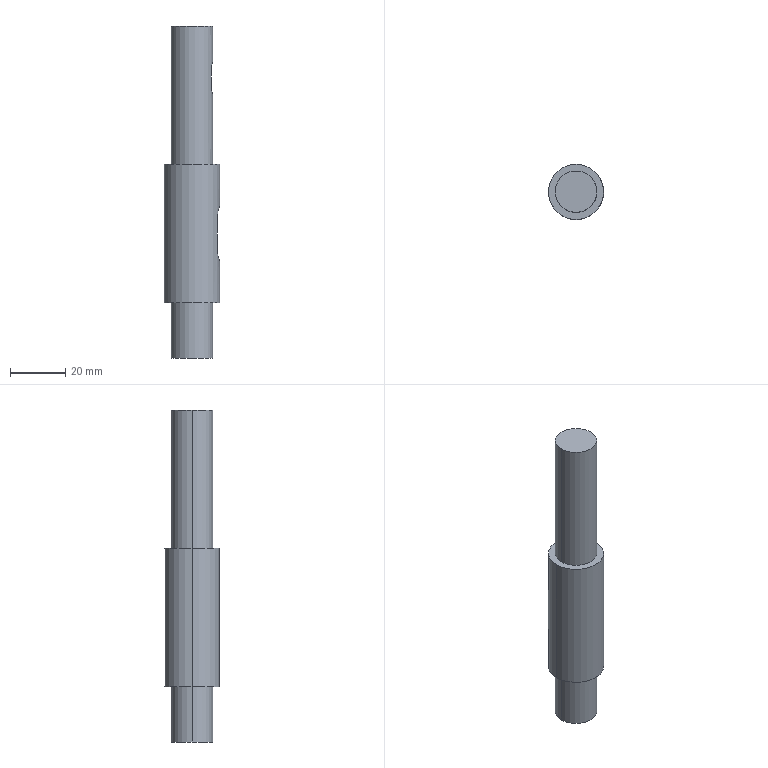Part | SolidWorks | features ICE 5, Extrusion 1 | 1 solid | 22 faces | box 20 x 20 x 120 mm | volume 27495 mm3 | cylinder 12 | plane 10 | commonest cylinder face diameters 15 x4 6 x3 8 x3 20 x2
STEP:
#1=CARTESIAN_POINT('',(-7.5,0.,-20.));
#2=VERTEX_POINT('',#1);
#3=CARTESIAN_POINT('',(7.5,0.,-20.));
#4=VERTEX_POINT('',#3);
#5=CARTESIAN_POINT('',(0.,0.,-20.));
#6=DIRECTION('',(0.,0.,-1.));
#7=DIRECTION('',(-1.,0.,0.));
#8=AXIS2_PLACEMENT_3D('',#5,#6,#7);
#9=CIRCLE('',#8,7.5);
#10=EDGE_CURVE('',#2,#4,#9,.T.);
#11=ORIENTED_EDGE('',*,*,#10,.F.);
#12=CARTESIAN_POINT('',(-7.5,0.,0.));
#13=VERTEX_POINT('',#12);
#14=CARTESIAN_POINT('',(-7.5,0.,-20.));
#15=DIRECTION('',(0.,0.,1.));
#16=VECTOR('',#15,1000.);
#17=LINE('',#14,#16);
#18=EDGE_CURVE('',#2,#13,#17,.T.);
#19=ORIENTED_EDGE('',*,*,#18,.T.);
#20=CARTESIAN_POINT('',(7.5,0.,0.));
#21=VERTEX_POINT('',#20);
#22=CARTESIAN_POINT('',(0.,0.,0.));
#23=DIRECTION('',(0.,0.,-1.));
#24=DIRECTION('',(-1.,0.,0.));
#25=AXIS2_PLACEMENT_3D('',#22,#23,#24);
#26=CIRCLE('',#25,7.5);
#27=EDGE_CURVE('',#13,#21,#26,.T.);
#28=ORIENTED_EDGE('',*,*,#27,.T.);
#29=CARTESIAN_POINT('',(7.5,0.,-20.));
#30=DIRECTION('',(0.,0.,1.));
#31=VECTOR('',#30,1000.);
#32=LINE('',#29,#31);
#33=EDGE_CURVE('',#4,#21,#32,.T.);
#34=ORIENTED_EDGE('',*,*,#33,.F.);
#35=EDGE_LOOP('',(#11,#19,#28,#34));
#36=FACE_OUTER_BOUND('',#35,.T.);
#37=CARTESIAN_POINT('',(0.,0.,-20.));
#38=DIRECTION('',(0.,0.,1.));
#39=DIRECTION('',(1.,0.,0.));
#40=AXIS2_PLACEMENT_3D('',#37,#38,#39);
#41=CYLINDRICAL_SURFACE('',#40,7.5);
#42=ADVANCED_FACE('',(#36),#41,.T.);
#43=CARTESIAN_POINT('',(4.5,0.,75.188));
#44=VERTEX_POINT('',#43);
#45=CARTESIAN_POINT('',(4.5,3.,78.188));
#46=VERTEX_POINT('',#45);
#47=CARTESIAN_POINT('',(4.5,0.,78.188));
#48=DIRECTION('',(1.,0.,0.));
#49=DIRECTION('',(0.,0.,-1.));
#50=AXIS2_PLACEMENT_3D('',#47,#48,#49);
#51=CIRCLE('',#50,3.);
#52=EDGE_CURVE('',#44,#46,#51,.T.);
#53=ORIENTED_EDGE('',*,*,#52,.F.);
#54=CARTESIAN_POINT('',(7.5,0.,75.188));
#55=VERTEX_POINT('',#54);
#56=CARTESIAN_POINT('',(4.5,0.,75.188));
#57=DIRECTION('',(1.,0.,0.));
#58=VECTOR('',#57,1000.);
#59=LINE('',#56,#58);
#60=EDGE_CURVE('',#44,#55,#59,.T.);
#61=ORIENTED_EDGE('',*,*,#60,.T.);
#62=CARTESIAN_POINT('',(6.874,3.,78.188));
#63=VERTEX_POINT('',#62);
#64=CARTESIAN_POINT('',(6.874,3.,78.188));
#65=CARTESIAN_POINT('',(6.874,3.,77.987));
#66=CARTESIAN_POINT('',(6.883,2.98,77.791));
#67=CARTESIAN_POINT('',(6.916,2.903,77.404));
#68=CARTESIAN_POINT('',(6.94,2.844,77.213));
#69=CARTESIAN_POINT('',(7.,2.693,76.851));
#70=CARTESIAN_POINT('',(7.036,2.6,76.679));
#71=CARTESIAN_POINT('',(7.112,2.383,76.355));
#72=CARTESIAN_POINT('',(7.154,2.258,76.203));
#73=CARTESIAN_POINT('',(7.275,1.847,75.792));
#74=CARTESIAN_POINT('',(7.354,1.515,75.57));
#75=CARTESIAN_POINT('',(7.439,0.9745,75.344));
#76=CARTESIAN_POINT('',(7.462,0.7831,75.285));
#77=CARTESIAN_POINT('',(7.492,0.3945,75.207));
#78=CARTESIAN_POINT('',(7.5,0.1982,75.188));
#79=CARTESIAN_POINT('',(7.5,0.,75.188));
#80=B_SPLINE_CURVE_WITH_KNOTS('',3,(#64,#65,#66,#67,#68,#69,#70,#71,#72,#73,#74,#75,#76,#77,#78,#79),.UNSPECIFIED.,.F.,.F.,(4,2,2,2,2,2,2,4),(0.,0.0005926,0.001185,0.001778,0.002371,0.003556,0.004148,0.004741),.UNSPECIFIED.);
#81=EDGE_CURVE('',#63,#55,#80,.T.);
#82=ORIENTED_EDGE('',*,*,#81,.F.);
#83=CARTESIAN_POINT('',(4.5,3.,78.188));
#84=DIRECTION('',(1.,0.,0.));
#85=VECTOR('',#84,1000.);
#86=LINE('',#83,#85);
#87=EDGE_CURVE('',#46,#63,#86,.T.);
#88=ORIENTED_EDGE('',*,*,#87,.F.);
#89=EDGE_LOOP('',(#53,#61,#82,#88));
#90=FACE_OUTER_BOUND('',#89,.T.);
#91=CARTESIAN_POINT('',(4.5,0.,78.188));
#92=DIRECTION('',(1.,0.,0.));
#93=DIRECTION('',(0.,0.,-1.));
#94=AXIS2_PLACEMENT_3D('',#91,#92,#93);
#95=CYLINDRICAL_SURFACE('',#94,3.);
#96=ADVANCED_FACE('',(#90),#95,.F.);
#97=CARTESIAN_POINT('',(7.5,0.,100.));
#98=VERTEX_POINT('',#97);
#99=CARTESIAN_POINT('',(-7.5,0.,100.));
#100=VERTEX_POINT('',#99);
#101=CARTESIAN_POINT('',(0.,0.,100.));
#102=DIRECTION('',(0.,0.,1.));
#103=DIRECTION('',(1.,0.,0.));
#104=AXIS2_PLACEMENT_3D('',#101,#102,#103);
#105=CIRCLE('',#104,7.5);
#106=EDGE_CURVE('',#98,#100,#105,.T.);
#107=ORIENTED_EDGE('',*,*,#106,.F.);
#108=CARTESIAN_POINT('',(7.5,0.,87.188));
#109=VERTEX_POINT('',#108);
#110=CARTESIAN_POINT('',(7.5,0.,100.));
#111=DIRECTION('',(0.,0.,-1.));
#112=VECTOR('',#111,1000.);
#113=LINE('',#110,#112);
#114=EDGE_CURVE('',#98,#109,#113,.T.);
#115=ORIENTED_EDGE('',*,*,#114,.T.);
#116=CARTESIAN_POINT('',(6.874,3.,84.188));
#117=VERTEX_POINT('',#116);
#118=CARTESIAN_POINT('',(7.5,0.,87.188));
#119=CARTESIAN_POINT('',(7.5,0.1979,87.188));
#120=CARTESIAN_POINT('',(7.492,0.3987,87.168));
#121=CARTESIAN_POINT('',(7.461,0.785,87.09));
#122=CARTESIAN_POINT('',(7.439,0.9732,87.033));
#123=CARTESIAN_POINT('',(7.382,1.339,86.88));
#124=CARTESIAN_POINT('',(7.348,1.51,86.787));
#125=CARTESIAN_POINT('',(7.274,1.833,86.571));
#126=CARTESIAN_POINT('',(7.234,1.985,86.445));
#127=CARTESIAN_POINT('',(7.153,2.26,86.171));
#128=CARTESIAN_POINT('',(7.113,2.382,86.022));
#129=CARTESIAN_POINT('',(7.036,2.599,85.698));
#130=CARTESIAN_POINT('',(7.,2.693,85.524));
#131=CARTESIAN_POINT('',(6.941,2.843,85.164));
#132=CARTESIAN_POINT('',(6.916,2.901,84.977));
#133=CARTESIAN_POINT('',(6.883,2.98,84.587));
#134=CARTESIAN_POINT('',(6.874,3.,84.388));
#135=CARTESIAN_POINT('',(6.874,3.,84.188));
#136=B_SPLINE_CURVE_WITH_KNOTS('',3,(#118,#119,#120,#121,#122,#123,#124,#125,#126,#127,#128,#129,#130,#131,#132,#133,#134,#135),.UNSPECIFIED.,.F.,.F.,(4,2,2,2,2,2,2,2,4),(0.004741,0.005333,0.005925,0.006516,0.007108,0.0077,0.008291,0.008883,0.009475),.UNSPECIFIED.);
#137=EDGE_CURVE('',#109,#117,#136,.T.);
#138=ORIENTED_EDGE('',*,*,#137,.T.);
#139=CARTESIAN_POINT('',(6.874,3.,100.));
#140=DIRECTION('',(0.,0.,-1.));
#141=VECTOR('',#140,1000.);
#142=LINE('',#139,#141);
#143=EDGE_CURVE('',#117,#63,#142,.T.);
#144=ORIENTED_EDGE('',*,*,#143,.T.);
#145=ORIENTED_EDGE('',*,*,#81,.T.);
#146=CARTESIAN_POINT('',(7.5,0.,50.));
#147=VERTEX_POINT('',#146);
#148=CARTESIAN_POINT('',(7.5,0.,100.));
#149=DIRECTION('',(0.,0.,-1.));
#150=VECTOR('',#149,1000.);
#151=LINE('',#148,#150);
#152=EDGE_CURVE('',#55,#147,#151,.T.);
#153=ORIENTED_EDGE('',*,*,#152,.T.);
#154=CARTESIAN_POINT('',(-7.5,0.,50.));
#155=VERTEX_POINT('',#154);
#156=CARTESIAN_POINT('',(0.,0.,50.));
#157=DIRECTION('',(0.,0.,1.));
#158=DIRECTION('',(1.,0.,0.));
#159=AXIS2_PLACEMENT_3D('',#156,#157,#158);
#160=CIRCLE('',#159,7.5);
#161=EDGE_CURVE('',#147,#155,#160,.T.);
#162=ORIENTED_EDGE('',*,*,#161,.T.);
#163=CARTESIAN_POINT('',(-7.5,0.,100.));
#164=DIRECTION('',(0.,0.,-1.));
#165=VECTOR('',#164,1000.);
#166=LINE('',#163,#165);
#167=EDGE_CURVE('',#100,#155,#166,.T.);
#168=ORIENTED_EDGE('',*,*,#167,.F.);
#169=EDGE_LOOP('',(#107,#115,#138,#144,#145,#153,#162,#168));
#170=FACE_OUTER_BOUND('',#169,.T.);
#171=CARTESIAN_POINT('',(0.,0.,100.));
#172=DIRECTION('',(0.,0.,-1.));
#173=DIRECTION('',(-1.,0.,0.));
#174=AXIS2_PLACEMENT_3D('',#171,#172,#173);
#175=CYLINDRICAL_SURFACE('',#174,7.5);
#176=ADVANCED_FACE('',(#170),#175,.T.);
#177=CARTESIAN_POINT('',(7.,0.,15.));
#178=VERTEX_POINT('',#177);
#179=CARTESIAN_POINT('',(7.,4.,19.));
#180=VERTEX_POINT('',#179);
#181=CARTESIAN_POINT('',(7.,0.,19.));
#182=DIRECTION('',(1.,0.,0.));
#183=DIRECTION('',(0.,0.,-1.));
#184=AXIS2_PLACEMENT_3D('',#181,#182,#183);
#185=CIRCLE('',#184,4.);
#186=EDGE_CURVE('',#178,#180,#185,.T.);
#187=ORIENTED_EDGE('',*,*,#186,.F.);
#188=CARTESIAN_POINT('',(10.,0.,15.));
#189=VERTEX_POINT('',#188);
#190=CARTESIAN_POINT('',(7.,0.,15.));
#191=DIRECTION('',(1.,0.,0.));
#192=VECTOR('',#191,1000.);
#193=LINE('',#190,#192);
#194=EDGE_CURVE('',#178,#189,#193,.T.);
#195=ORIENTED_EDGE('',*,*,#194,.T.);
#196=CARTESIAN_POINT('',(9.165,4.,19.));
#197=VERTEX_POINT('',#196);
#198=CARTESIAN_POINT('',(9.165,4.,19.));
#199=CARTESIAN_POINT('',(9.165,4.,18.733));
#200=CARTESIAN_POINT('',(9.177,3.973,18.47));
#201=CARTESIAN_POINT('',(9.221,3.87,17.955));
#202=CARTESIAN_POINT('',(9.254,3.792,17.7));
#203=CARTESIAN_POINT('',(9.334,3.59,17.217));
#204=CARTESIAN_POINT('',(9.381,3.467,16.988));
#205=CARTESIAN_POINT('',(9.483,3.177,16.555));
#206=CARTESIAN_POINT('',(9.538,3.01,16.353));
#207=CARTESIAN_POINT('',(9.646,2.645,15.988));
#208=CARTESIAN_POINT('',(9.699,2.444,15.823));
#209=CARTESIAN_POINT('',(9.799,2.009,15.531));
#210=CARTESIAN_POINT('',(9.843,1.78,15.409));
#211=CARTESIAN_POINT('',(9.918,1.299,15.208));
#212=CARTESIAN_POINT('',(9.949,1.044,15.13));
#213=CARTESIAN_POINT('',(9.99,0.526,15.026));
#214=CARTESIAN_POINT('',(10.,0.2643,15.));
#215=CARTESIAN_POINT('',(10.,0.,15.));
#216=B_SPLINE_CURVE_WITH_KNOTS('',3,(#198,#199,#200,#201,#202,#203,#204,#205,#206,#207,#208,#209,#210,#211,#212,#213,#214,#215),.UNSPECIFIED.,.F.,.F.,(4,2,2,2,2,2,2,2,4),(0.,0.0007902,0.00158,0.002371,0.003161,0.003951,0.004741,0.005531,0.006322),.UNSPECIFIED.);
#217=EDGE_CURVE('',#197,#189,#216,.T.);
#218=ORIENTED_EDGE('',*,*,#217,.F.);
#219=CARTESIAN_POINT('',(7.,4.,19.));
#220=DIRECTION('',(1.,0.,0.));
#221=VECTOR('',#220,1000.);
#222=LINE('',#219,#221);
#223=EDGE_CURVE('',#180,#197,#222,.T.);
#224=ORIENTED_EDGE('',*,*,#223,.F.);
#225=EDGE_LOOP('',(#187,#195,#218,#224));
#226=FACE_OUTER_BOUND('',#225,.T.);
#227=CARTESIAN_POINT('',(7.,0.,19.));
#228=DIRECTION('',(1.,0.,0.));
#229=DIRECTION('',(0.,0.,-1.));
#230=AXIS2_PLACEMENT_3D('',#227,#228,#229);
#231=CYLINDRICAL_SURFACE('',#230,4.);
#232=ADVANCED_FACE('',(#226),#231,.F.);
#233=CARTESIAN_POINT('',(10.,0.,50.));
#234=VERTEX_POINT('',#233);
#235=CARTESIAN_POINT('',(-10.,0.,50.));
#236=VERTEX_POINT('',#235);
#237=CARTESIAN_POINT('',(0.,0.,50.));
#238=DIRECTION('',(0.,0.,1.));
#239=DIRECTION('',(1.,0.,0.));
#240=AXIS2_PLACEMENT_3D('',#237,#238,#239);
#241=CIRCLE('',#240,10.);
#242=EDGE_CURVE('',#234,#236,#241,.T.);
#243=ORIENTED_EDGE('',*,*,#242,.F.);
#244=CARTESIAN_POINT('',(10.,0.,35.));
#245=VERTEX_POINT('',#244);
#246=CARTESIAN_POINT('',(10.,0.,60.));
#247=DIRECTION('',(0.,0.,-1.));
#248=VECTOR('',#247,1000.);
#249=LINE('',#246,#248);
#250=EDGE_CURVE('',#234,#245,#249,.T.);
#251=ORIENTED_EDGE('',*,*,#250,.T.);
#252=CARTESIAN_POINT('',(9.165,4.,31.));
#253=VERTEX_POINT('',#252);
#254=CARTESIAN_POINT('',(10.,0.,35.));
#255=CARTESIAN_POINT('',(10.,0.2639,35.));
#256=CARTESIAN_POINT('',(9.989,0.5316,34.973));
#257=CARTESIAN_POINT('',(9.948,1.047,34.87));
#258=CARTESIAN_POINT('',(9.919,1.298,34.793));
#259=CARTESIAN_POINT('',(9.843,1.785,34.589));
#260=CARTESIAN_POINT('',(9.798,2.014,34.466));
#261=CARTESIAN_POINT('',(9.699,2.444,34.177));
#262=CARTESIAN_POINT('',(9.645,2.647,34.01));
#263=CARTESIAN_POINT('',(9.537,3.013,33.644));
#264=CARTESIAN_POINT('',(9.483,3.176,33.445));
#265=CARTESIAN_POINT('',(9.381,3.466,33.014));
#266=CARTESIAN_POINT('',(9.334,3.591,32.781));
#267=CARTESIAN_POINT('',(9.254,3.791,32.302));
#268=CARTESIAN_POINT('',(9.222,3.868,32.052));
#269=CARTESIAN_POINT('',(9.177,3.973,31.533));
#270=CARTESIAN_POINT('',(9.165,4.,31.267));
#271=CARTESIAN_POINT('',(9.165,4.,31.));
#272=B_SPLINE_CURVE_WITH_KNOTS('',3,(#254,#255,#256,#257,#258,#259,#260,#261,#262,#263,#264,#265,#266,#267,#268,#269,#270,#271),.UNSPECIFIED.,.F.,.F.,(4,2,2,2,2,2,2,2,4),(0.006322,0.00711,0.007899,0.008688,0.009477,0.01027,0.01106,0.01184,0.01263),.UNSPECIFIED.);
#273=EDGE_CURVE('',#245,#253,#272,.T.);
#274=ORIENTED_EDGE('',*,*,#273,.T.);
#275=CARTESIAN_POINT('',(9.165,4.,60.));
#276=DIRECTION('',(0.,0.,-1.));
#277=VECTOR('',#276,1000.);
#278=LINE('',#275,#277);
#279=EDGE_CURVE('',#253,#197,#278,.T.);
#280=ORIENTED_EDGE('',*,*,#279,.T.);
#281=ORIENTED_EDGE('',*,*,#217,.T.);
#282=CARTESIAN_POINT('',(10.,0.,0.));
#283=VERTEX_POINT('',#282);
#284=CARTESIAN_POINT('',(10.,0.,60.));
#285=DIRECTION('',(0.,0.,-1.));
#286=VECTOR('',#285,1000.);
#287=LINE('',#284,#286);
#288=EDGE_CURVE('',#189,#283,#287,.T.);
#289=ORIENTED_EDGE('',*,*,#288,.T.);
#290=CARTESIAN_POINT('',(-10.,0.,0.));
#291=VERTEX_POINT('',#290);
#292=CARTESIAN_POINT('',(0.,0.,0.));
#293=DIRECTION('',(0.,0.,1.));
#294=DIRECTION('',(1.,0.,0.));
#295=AXIS2_PLACEMENT_3D('',#292,#293,#294);
#296=CIRCLE('',#295,10.);
#297=EDGE_CURVE('',#283,#291,#296,.T.);
#298=ORIENTED_EDGE('',*,*,#297,.T.);
#299=CARTESIAN_POINT('',(-10.,0.,60.));
#300=DIRECTION('',(0.,0.,-1.));
#301=VECTOR('',#300,1000.);
#302=LINE('',#299,#301);
#303=EDGE_CURVE('',#236,#291,#302,.T.);
#304=ORIENTED_EDGE('',*,*,#303,.F.);
#305=EDGE_LOOP('',(#243,#251,#274,#280,#281,#289,#298,#304));
#306=FACE_OUTER_BOUND('',#305,.T.);
#307=CARTESIAN_POINT('',(0.,0.,60.));
#308=DIRECTION('',(0.,0.,-1.));
#309=DIRECTION('',(-1.,0.,0.));
#310=AXIS2_PLACEMENT_3D('',#307,#308,#309);
#311=CYLINDRICAL_SURFACE('',#310,10.);
#312=ADVANCED_FACE('',(#306),#311,.T.);
#313=ORIENTED_EDGE('',*,*,#250,.F.);
#314=CARTESIAN_POINT('',(0.,0.,50.));
#315=DIRECTION('',(0.,0.,1.));
#316=DIRECTION('',(1.,0.,0.));
#317=AXIS2_PLACEMENT_3D('',#314,#315,#316);
#318=CIRCLE('',#317,10.);
#319=EDGE_CURVE('',#236,#234,#318,.T.);
#320=ORIENTED_EDGE('',*,*,#319,.F.);
#321=ORIENTED_EDGE('',*,*,#303,.T.);
#322=CARTESIAN_POINT('',(0.,0.,0.));
#323=DIRECTION('',(0.,0.,1.));
#324=DIRECTION('',(1.,0.,0.));
#325=AXIS2_PLACEMENT_3D('',#322,#323,#324);
#326=CIRCLE('',#325,10.);
#327=EDGE_CURVE('',#291,#283,#326,.T.);
#328=ORIENTED_EDGE('',*,*,#327,.T.);
#329=ORIENTED_EDGE('',*,*,#288,.F.);
#330=CARTESIAN_POINT('',(9.165,-4.,19.));
#331=VERTEX_POINT('',#330);
#332=CARTESIAN_POINT('',(10.,0.,15.));
#333=CARTESIAN_POINT('',(10.,-0.2639,15.));
#334=CARTESIAN_POINT('',(9.989,-0.5316,15.027));
#335=CARTESIAN_POINT('',(9.948,-1.047,15.13));
#336=CARTESIAN_POINT('',(9.919,-1.298,15.207));
#337=CARTESIAN_POINT('',(9.843,-1.785,15.411));
#338=CARTESIAN_POINT('',(9.798,-2.014,15.534));
#339=CARTESIAN_POINT('',(9.699,-2.444,15.823));
#340=CARTESIAN_POINT('',(9.645,-2.647,15.99));
#341=CARTESIAN_POINT('',(9.537,-3.013,16.356));
#342=CARTESIAN_POINT('',(9.483,-3.176,16.555));
#343=CARTESIAN_POINT('',(9.381,-3.466,16.986));
#344=CARTESIAN_POINT('',(9.334,-3.591,17.219));
#345=CARTESIAN_POINT('',(9.254,-3.791,17.698));
#346=CARTESIAN_POINT('',(9.222,-3.868,17.948));
#347=CARTESIAN_POINT('',(9.177,-3.973,18.467));
#348=CARTESIAN_POINT('',(9.165,-4.,18.733));
#349=CARTESIAN_POINT('',(9.165,-4.,19.));
#350=B_SPLINE_CURVE_WITH_KNOTS('',3,(#332,#333,#334,#335,#336,#337,#338,#339,#340,#341,#342,#343,#344,#345,#346,#347,#348,#349),.UNSPECIFIED.,.F.,.F.,(4,2,2,2,2,2,2,2,4),(0.006322,0.00711,0.007899,0.008688,0.009477,0.01027,0.01106,0.01184,0.01263),.UNSPECIFIED.);
#351=EDGE_CURVE('',#189,#331,#350,.T.);
#352=ORIENTED_EDGE('',*,*,#351,.T.);
#353=CARTESIAN_POINT('',(9.165,-4.,31.));
#354=VERTEX_POINT('',#353);
#355=CARTESIAN_POINT('',(9.165,-4.,60.));
#356=DIRECTION('',(0.,0.,1.));
#357=VECTOR('',#356,1000.);
#358=LINE('',#355,#357);
#359=EDGE_CURVE('',#331,#354,#358,.T.);
#360=ORIENTED_EDGE('',*,*,#359,.T.);
#361=CARTESIAN_POINT('',(9.165,-4.,31.));
#362=CARTESIAN_POINT('',(9.165,-4.,31.267));
#363=CARTESIAN_POINT('',(9.177,-3.973,31.53));
#364=CARTESIAN_POINT('',(9.221,-3.87,32.045));
#365=CARTESIAN_POINT('',(9.254,-3.792,32.3));
#366=CARTESIAN_POINT('',(9.334,-3.59,32.783));
#367=CARTESIAN_POINT('',(9.381,-3.467,33.012));
#368=CARTESIAN_POINT('',(9.483,-3.177,33.445));
#369=CARTESIAN_POINT('',(9.538,-3.01,33.647));
#370=CARTESIAN_POINT('',(9.646,-2.645,34.012));
#371=CARTESIAN_POINT('',(9.699,-2.444,34.177));
#372=CARTESIAN_POINT('',(9.799,-2.009,34.469));
#373=CARTESIAN_POINT('',(9.843,-1.78,34.591));
#374=CARTESIAN_POINT('',(9.918,-1.299,34.792));
#375=CARTESIAN_POINT('',(9.949,-1.044,34.87));
#376=CARTESIAN_POINT('',(9.99,-0.526,34.974));
#377=CARTESIAN_POINT('',(10.,-0.2643,35.));
#378=CARTESIAN_POINT('',(10.,0.,35.));
#379=B_SPLINE_CURVE_WITH_KNOTS('',3,(#361,#362,#363,#364,#365,#366,#367,#368,#369,#370,#371,#372,#373,#374,#375,#376,#377,#378),.UNSPECIFIED.,.F.,.F.,(4,2,2,2,2,2,2,2,4),(0.,0.0007902,0.00158,0.002371,0.003161,0.003951,0.004741,0.005531,0.006322),.UNSPECIFIED.);
#380=EDGE_CURVE('',#354,#245,#379,.T.);
#381=ORIENTED_EDGE('',*,*,#380,.T.);
#382=EDGE_LOOP('',(#313,#320,#321,#328,#329,#352,#360,#381));
#383=FACE_OUTER_BOUND('',#382,.T.);
#384=CARTESIAN_POINT('',(0.,0.,60.));
#385=DIRECTION('',(0.,0.,-1.));
#386=DIRECTION('',(-1.,0.,0.));
#387=AXIS2_PLACEMENT_3D('',#384,#385,#386);
#388=CYLINDRICAL_SURFACE('',#387,10.);
#389=ADVANCED_FACE('',(#383),#388,.T.);
#390=CARTESIAN_POINT('',(0.,0.,0.));
#391=DIRECTION('',(0.,0.,-1.));
#392=DIRECTION('',(-1.,0.,0.));
#393=AXIS2_PLACEMENT_3D('',#390,#391,#392);
#394=CIRCLE('',#393,7.5);
#395=EDGE_CURVE('',#21,#13,#394,.T.);
#396=ORIENTED_EDGE('',*,*,#395,.F.);
#397=ORIENTED_EDGE('',*,*,#27,.F.);
#398=EDGE_LOOP('',(#396,#397));
#399=FACE_BOUND('',#398,.T.);
#400=ORIENTED_EDGE('',*,*,#327,.F.);
#401=ORIENTED_EDGE('',*,*,#297,.F.);
#402=EDGE_LOOP('',(#400,#401));
#403=FACE_OUTER_BOUND('',#402,.T.);
#404=CARTESIAN_POINT('',(0.,0.,0.));
#405=DIRECTION('',(0.,0.,1.));
#406=DIRECTION('',(1.,0.,0.));
#407=AXIS2_PLACEMENT_3D('',#404,#405,#406);
#408=PLANE('',#407);
#409=ADVANCED_FACE('',(#399,#403),#408,.F.);
#410=CARTESIAN_POINT('',(7.,-4.,31.));
#411=VERTEX_POINT('',#410);
#412=CARTESIAN_POINT('',(7.,-4.,31.));
#413=DIRECTION('',(1.,0.,0.));
#414=VECTOR('',#413,1000.);
#415=LINE('',#412,#414);
#416=EDGE_CURVE('',#411,#354,#415,.T.);
#417=ORIENTED_EDGE('',*,*,#416,.F.);
#418=CARTESIAN_POINT('',(7.,4.,31.));
#419=VERTEX_POINT('',#418);
#420=CARTESIAN_POINT('',(7.,0.,31.));
#421=DIRECTION('',(1.,0.,0.));
#422=DIRECTION('',(0.,0.,-1.));
#423=AXIS2_PLACEMENT_3D('',#420,#421,#422);
#424=CIRCLE('',#423,4.);
#425=EDGE_CURVE('',#419,#411,#424,.T.);
#426=ORIENTED_EDGE('',*,*,#425,.F.);
#427=CARTESIAN_POINT('',(7.,4.,31.));
#428=DIRECTION('',(1.,0.,0.));
#429=VECTOR('',#428,1000.);
#430=LINE('',#427,#429);
#431=EDGE_CURVE('',#419,#253,#430,.T.);
#432=ORIENTED_EDGE('',*,*,#431,.T.);
#433=ORIENTED_EDGE('',*,*,#273,.F.);
#434=ORIENTED_EDGE('',*,*,#380,.F.);
#435=EDGE_LOOP('',(#417,#426,#432,#433,#434));
#436=FACE_OUTER_BOUND('',#435,.T.);
#437=CARTESIAN_POINT('',(7.,0.,31.));
#438=DIRECTION('',(1.,0.,0.));
#439=DIRECTION('',(0.,0.,-1.));
#440=AXIS2_PLACEMENT_3D('',#437,#438,#439);
#441=CYLINDRICAL_SURFACE('',#440,4.);
#442=ADVANCED_FACE('',(#436),#441,.F.);
#443=ORIENTED_EDGE('',*,*,#431,.F.);
#444=CARTESIAN_POINT('',(7.,4.,31.));
#445=DIRECTION('',(0.,0.,1.));
#446=VECTOR('',#445,1000.);
#447=LINE('',#444,#446);
#448=EDGE_CURVE('',#180,#419,#447,.T.);
#449=ORIENTED_EDGE('',*,*,#448,.F.);
#450=ORIENTED_EDGE('',*,*,#223,.T.);
#451=ORIENTED_EDGE('',*,*,#279,.F.);
#452=EDGE_LOOP('',(#443,#449,#450,#451));
#453=FACE_OUTER_BOUND('',#452,.T.);
#454=CARTESIAN_POINT('',(7.,4.,31.));
#455=DIRECTION('',(0.,1.,0.));
#456=DIRECTION('',(0.,0.,1.));
#457=AXIS2_PLACEMENT_3D('',#454,#455,#456);
#458=PLANE('',#457);
#459=ADVANCED_FACE('',(#453),#458,.F.);
#460=ORIENTED_EDGE('',*,*,#194,.F.);
#461=CARTESIAN_POINT('',(7.,-4.,19.));
#462=VERTEX_POINT('',#461);
#463=CARTESIAN_POINT('',(7.,0.,19.));
#464=DIRECTION('',(1.,0.,0.));
#465=DIRECTION('',(0.,0.,-1.));
#466=AXIS2_PLACEMENT_3D('',#463,#464,#465);
#467=CIRCLE('',#466,4.);
#468=EDGE_CURVE('',#462,#178,#467,.T.);
#469=ORIENTED_EDGE('',*,*,#468,.F.);
#470=CARTESIAN_POINT('',(7.,-4.,19.));
#471=DIRECTION('',(1.,0.,0.));
#472=VECTOR('',#471,1000.);
#473=LINE('',#470,#472);
#474=EDGE_CURVE('',#462,#331,#473,.T.);
#475=ORIENTED_EDGE('',*,*,#474,.T.);
#476=ORIENTED_EDGE('',*,*,#351,.F.);
#477=EDGE_LOOP('',(#460,#469,#475,#476));
#478=FACE_OUTER_BOUND('',#477,.T.);
#479=CARTESIAN_POINT('',(7.,0.,19.));
#480=DIRECTION('',(1.,0.,0.));
#481=DIRECTION('',(0.,0.,-1.));
#482=AXIS2_PLACEMENT_3D('',#479,#480,#481);
#483=CYLINDRICAL_SURFACE('',#482,4.);
#484=ADVANCED_FACE('',(#478),#483,.F.);
#485=ORIENTED_EDGE('',*,*,#474,.F.);
#486=CARTESIAN_POINT('',(7.,-4.,31.));
#487=DIRECTION('',(0.,0.,-1.));
#488=VECTOR('',#487,1000.);
#489=LINE('',#486,#488);
#490=EDGE_CURVE('',#411,#462,#489,.T.);
#491=ORIENTED_EDGE('',*,*,#490,.F.);
#492=ORIENTED_EDGE('',*,*,#416,.T.);
#493=ORIENTED_EDGE('',*,*,#359,.F.);
#494=EDGE_LOOP('',(#485,#491,#492,#493));
#495=FACE_OUTER_BOUND('',#494,.T.);
#496=CARTESIAN_POINT('',(7.,-4.,31.));
#497=DIRECTION('',(0.,-1.,0.));
#498=DIRECTION('',(0.,0.,-1.));
#499=AXIS2_PLACEMENT_3D('',#496,#497,#498);
#500=PLANE('',#499);
#501=ADVANCED_FACE('',(#495),#500,.F.);
#502=ORIENTED_EDGE('',*,*,#425,.T.);
#503=ORIENTED_EDGE('',*,*,#490,.T.);
#504=ORIENTED_EDGE('',*,*,#468,.T.);
#505=ORIENTED_EDGE('',*,*,#186,.T.);
#506=ORIENTED_EDGE('',*,*,#448,.T.);
#507=EDGE_LOOP('',(#502,#503,#504,#505,#506));
#508=FACE_OUTER_BOUND('',#507,.T.);
#509=CARTESIAN_POINT('',(7.,0.,31.));
#510=DIRECTION('',(1.,0.,0.));
#511=DIRECTION('',(0.,0.,-1.));
#512=AXIS2_PLACEMENT_3D('',#509,#510,#511);
#513=PLANE('',#512);
#514=ADVANCED_FACE('',(#508),#513,.T.);
#515=CARTESIAN_POINT('',(0.,0.,50.));
#516=DIRECTION('',(0.,0.,1.));
#517=DIRECTION('',(1.,0.,0.));
#518=AXIS2_PLACEMENT_3D('',#515,#516,#517);
#519=CIRCLE('',#518,7.5);
#520=EDGE_CURVE('',#155,#147,#519,.T.);
#521=ORIENTED_EDGE('',*,*,#520,.F.);
#522=ORIENTED_EDGE('',*,*,#161,.F.);
#523=EDGE_LOOP('',(#521,#522));
#524=FACE_BOUND('',#523,.T.);
#525=ORIENTED_EDGE('',*,*,#319,.T.);
#526=ORIENTED_EDGE('',*,*,#242,.T.);
#527=EDGE_LOOP('',(#525,#526));
#528=FACE_OUTER_BOUND('',#527,.T.);
#529=CARTESIAN_POINT('',(0.,0.,50.));
#530=DIRECTION('',(0.,0.,1.));
#531=DIRECTION('',(1.,0.,0.));
#532=AXIS2_PLACEMENT_3D('',#529,#530,#531);
#533=PLANE('',#532);
#534=ADVANCED_FACE('',(#524,#528),#533,.T.);
#535=CARTESIAN_POINT('',(0.,0.,100.));
#536=DIRECTION('',(0.,0.,1.));
#537=DIRECTION('',(1.,0.,0.));
#538=AXIS2_PLACEMENT_3D('',#535,#536,#537);
#539=CIRCLE('',#538,7.5);
#540=EDGE_CURVE('',#100,#98,#539,.T.);
#541=ORIENTED_EDGE('',*,*,#540,.T.);
#542=ORIENTED_EDGE('',*,*,#106,.T.);
#543=EDGE_LOOP('',(#541,#542));
#544=FACE_OUTER_BOUND('',#543,.T.);
#545=CARTESIAN_POINT('',(0.,0.,100.));
#546=DIRECTION('',(0.,0.,1.));
#547=DIRECTION('',(1.,0.,0.));
#548=AXIS2_PLACEMENT_3D('',#545,#546,#547);
#549=PLANE('',#548);
#550=ADVANCED_FACE('',(#544),#549,.T.);
#551=ORIENTED_EDGE('',*,*,#114,.F.);
#552=ORIENTED_EDGE('',*,*,#540,.F.);
#553=ORIENTED_EDGE('',*,*,#167,.T.);
#554=ORIENTED_EDGE('',*,*,#520,.T.);
#555=ORIENTED_EDGE('',*,*,#152,.F.);
#556=CARTESIAN_POINT('',(6.874,-3.,78.188));
#557=VERTEX_POINT('',#556);
#558=CARTESIAN_POINT('',(7.5,0.,75.188));
#559=CARTESIAN_POINT('',(7.5,-0.1979,75.188));
#560=CARTESIAN_POINT('',(7.492,-0.3987,75.208));
#561=CARTESIAN_POINT('',(7.461,-0.785,75.286));
#562=CARTESIAN_POINT('',(7.439,-0.9732,75.343));
#563=CARTESIAN_POINT('',(7.382,-1.339,75.496));
#564=CARTESIAN_POINT('',(7.348,-1.51,75.589));
#565=CARTESIAN_POINT('',(7.274,-1.833,75.805));
#566=CARTESIAN_POINT('',(7.234,-1.985,75.931));
#567=CARTESIAN_POINT('',(7.153,-2.26,76.205));
#568=CARTESIAN_POINT('',(7.113,-2.382,76.354));
#569=CARTESIAN_POINT('',(7.036,-2.599,76.678));
#570=CARTESIAN_POINT('',(7.,-2.693,76.852));
#571=CARTESIAN_POINT('',(6.941,-2.843,77.212));
#572=CARTESIAN_POINT('',(6.916,-2.901,77.399));
#573=CARTESIAN_POINT('',(6.883,-2.98,77.789));
#574=CARTESIAN_POINT('',(6.874,-3.,77.988));
#575=CARTESIAN_POINT('',(6.874,-3.,78.188));
#576=B_SPLINE_CURVE_WITH_KNOTS('',3,(#558,#559,#560,#561,#562,#563,#564,#565,#566,#567,#568,#569,#570,#571,#572,#573,#574,#575),.UNSPECIFIED.,.F.,.F.,(4,2,2,2,2,2,2,2,4),(0.004741,0.005333,0.005925,0.006516,0.007108,0.0077,0.008291,0.008883,0.009475),.UNSPECIFIED.);
#577=EDGE_CURVE('',#55,#557,#576,.T.);
#578=ORIENTED_EDGE('',*,*,#577,.T.);
#579=CARTESIAN_POINT('',(6.874,-3.,84.188));
#580=VERTEX_POINT('',#579);
#581=CARTESIAN_POINT('',(6.874,-3.,100.));
#582=DIRECTION('',(0.,0.,1.));
#583=VECTOR('',#582,1000.);
#584=LINE('',#581,#583);
#585=EDGE_CURVE('',#557,#580,#584,.T.);
#586=ORIENTED_EDGE('',*,*,#585,.T.);
#587=CARTESIAN_POINT('',(6.874,-3.,84.188));
#588=CARTESIAN_POINT('',(6.874,-3.,84.389));
#589=CARTESIAN_POINT('',(6.883,-2.98,84.585));
#590=CARTESIAN_POINT('',(6.916,-2.903,84.972));
#591=CARTESIAN_POINT('',(6.94,-2.844,85.163));
#592=CARTESIAN_POINT('',(7.,-2.693,85.525));
#593=CARTESIAN_POINT('',(7.036,-2.6,85.697));
#594=CARTESIAN_POINT('',(7.112,-2.383,86.021));
#595=CARTESIAN_POINT('',(7.154,-2.258,86.173));
#596=CARTESIAN_POINT('',(7.275,-1.847,86.584));
#597=CARTESIAN_POINT('',(7.354,-1.515,86.806));
#598=CARTESIAN_POINT('',(7.439,-0.9745,87.032));
#599=CARTESIAN_POINT('',(7.462,-0.7831,87.091));
#600=CARTESIAN_POINT('',(7.492,-0.3945,87.169));
#601=CARTESIAN_POINT('',(7.5,-0.1982,87.188));
#602=CARTESIAN_POINT('',(7.5,0.,87.188));
#603=B_SPLINE_CURVE_WITH_KNOTS('',3,(#587,#588,#589,#590,#591,#592,#593,#594,#595,#596,#597,#598,#599,#600,#601,#602),.UNSPECIFIED.,.F.,.F.,(4,2,2,2,2,2,2,4),(0.,0.0005926,0.001185,0.001778,0.002371,0.003556,0.004148,0.004741),.UNSPECIFIED.);
#604=EDGE_CURVE('',#580,#109,#603,.T.);
#605=ORIENTED_EDGE('',*,*,#604,.T.);
#606=EDGE_LOOP('',(#551,#552,#553,#554,#555,#578,#586,#605));
#607=FACE_OUTER_BOUND('',#606,.T.);
#608=CARTESIAN_POINT('',(0.,0.,100.));
#609=DIRECTION('',(0.,0.,-1.));
#610=DIRECTION('',(-1.,0.,0.));
#611=AXIS2_PLACEMENT_3D('',#608,#609,#610);
#612=CYLINDRICAL_SURFACE('',#611,7.5);
#613=ADVANCED_FACE('',(#607),#612,.T.);
#614=CARTESIAN_POINT('',(4.5,-3.,84.188));
#615=VERTEX_POINT('',#614);
#616=CARTESIAN_POINT('',(4.5,-3.,84.188));
#617=DIRECTION('',(1.,0.,0.));
#618=VECTOR('',#617,1000.);
#619=LINE('',#616,#618);
#620=EDGE_CURVE('',#615,#580,#619,.T.);
#621=ORIENTED_EDGE('',*,*,#620,.F.);
#622=CARTESIAN_POINT('',(4.5,3.,84.188));
#623=VERTEX_POINT('',#622);
#624=CARTESIAN_POINT('',(4.5,0.,84.188));
#625=DIRECTION('',(1.,0.,0.));
#626=DIRECTION('',(0.,0.,-1.));
#627=AXIS2_PLACEMENT_3D('',#624,#625,#626);
#628=CIRCLE('',#627,3.);
#629=EDGE_CURVE('',#623,#615,#628,.T.);
#630=ORIENTED_EDGE('',*,*,#629,.F.);
#631=CARTESIAN_POINT('',(4.5,3.,84.188));
#632=DIRECTION('',(1.,0.,0.));
#633=VECTOR('',#632,1000.);
#634=LINE('',#631,#633);
#635=EDGE_CURVE('',#623,#117,#634,.T.);
#636=ORIENTED_EDGE('',*,*,#635,.T.);
#637=ORIENTED_EDGE('',*,*,#137,.F.);
#638=ORIENTED_EDGE('',*,*,#604,.F.);
#639=EDGE_LOOP('',(#621,#630,#636,#637,#638));
#640=FACE_OUTER_BOUND('',#639,.T.);
#641=CARTESIAN_POINT('',(4.5,0.,84.188));
#642=DIRECTION('',(1.,0.,0.));
#643=DIRECTION('',(0.,0.,-1.));
#644=AXIS2_PLACEMENT_3D('',#641,#642,#643);
#645=CYLINDRICAL_SURFACE('',#644,3.);
#646=ADVANCED_FACE('',(#640),#645,.F.);
#647=ORIENTED_EDGE('',*,*,#635,.F.);
#648=CARTESIAN_POINT('',(4.5,3.,84.188));
#649=DIRECTION('',(0.,0.,1.));
#650=VECTOR('',#649,1000.);
#651=LINE('',#648,#650);
#652=EDGE_CURVE('',#46,#623,#651,.T.);
#653=ORIENTED_EDGE('',*,*,#652,.F.);
#654=ORIENTED_EDGE('',*,*,#87,.T.);
#655=ORIENTED_EDGE('',*,*,#143,.F.);
#656=EDGE_LOOP('',(#647,#653,#654,#655));
#657=FACE_OUTER_BOUND('',#656,.T.);
#658=CARTESIAN_POINT('',(4.5,3.,84.188));
#659=DIRECTION('',(0.,1.,0.));
#660=DIRECTION('',(0.,0.,1.));
#661=AXIS2_PLACEMENT_3D('',#658,#659,#660);
#662=PLANE('',#661);
#663=ADVANCED_FACE('',(#657),#662,.F.);
#664=ORIENTED_EDGE('',*,*,#60,.F.);
#665=CARTESIAN_POINT('',(4.5,-3.,78.188));
#666=VERTEX_POINT('',#665);
#667=CARTESIAN_POINT('',(4.5,0.,78.188));
#668=DIRECTION('',(1.,0.,0.));
#669=DIRECTION('',(0.,0.,-1.));
#670=AXIS2_PLACEMENT_3D('',#667,#668,#669);
#671=CIRCLE('',#670,3.);
#672=EDGE_CURVE('',#666,#44,#671,.T.);
#673=ORIENTED_EDGE('',*,*,#672,.F.);
#674=CARTESIAN_POINT('',(4.5,-3.,78.188));
#675=DIRECTION('',(1.,0.,0.));
#676=VECTOR('',#675,1000.);
#677=LINE('',#674,#676);
#678=EDGE_CURVE('',#666,#557,#677,.T.);
#679=ORIENTED_EDGE('',*,*,#678,.T.);
#680=ORIENTED_EDGE('',*,*,#577,.F.);
#681=EDGE_LOOP('',(#664,#673,#679,#680));
#682=FACE_OUTER_BOUND('',#681,.T.);
#683=CARTESIAN_POINT('',(4.5,0.,78.188));
#684=DIRECTION('',(1.,0.,0.));
#685=DIRECTION('',(0.,0.,-1.));
#686=AXIS2_PLACEMENT_3D('',#683,#684,#685);
#687=CYLINDRICAL_SURFACE('',#686,3.);
#688=ADVANCED_FACE('',(#682),#687,.F.);
#689=ORIENTED_EDGE('',*,*,#678,.F.);
#690=CARTESIAN_POINT('',(4.5,-3.,84.188));
#691=DIRECTION('',(0.,0.,-1.));
#692=VECTOR('',#691,1000.);
#693=LINE('',#690,#692);
#694=EDGE_CURVE('',#615,#666,#693,.T.);
#695=ORIENTED_EDGE('',*,*,#694,.F.);
#696=ORIENTED_EDGE('',*,*,#620,.T.);
#697=ORIENTED_EDGE('',*,*,#585,.F.);
#698=EDGE_LOOP('',(#689,#695,#696,#697));
#699=FACE_OUTER_BOUND('',#698,.T.);
#700=CARTESIAN_POINT('',(4.5,-3.,84.188));
#701=DIRECTION('',(0.,-1.,0.));
#702=DIRECTION('',(0.,0.,-1.));
#703=AXIS2_PLACEMENT_3D('',#700,#701,#702);
#704=PLANE('',#703);
#705=ADVANCED_FACE('',(#699),#704,.F.);
#706=ORIENTED_EDGE('',*,*,#629,.T.);
#707=ORIENTED_EDGE('',*,*,#694,.T.);
#708=ORIENTED_EDGE('',*,*,#672,.T.);
#709=ORIENTED_EDGE('',*,*,#52,.T.);
#710=ORIENTED_EDGE('',*,*,#652,.T.);
#711=EDGE_LOOP('',(#706,#707,#708,#709,#710));
#712=FACE_OUTER_BOUND('',#711,.T.);
#713=CARTESIAN_POINT('',(4.5,0.,84.188));
#714=DIRECTION('',(1.,0.,0.));
#715=DIRECTION('',(0.,0.,-1.));
#716=AXIS2_PLACEMENT_3D('',#713,#714,#715);
#717=PLANE('',#716);
#718=ADVANCED_FACE('',(#712),#717,.T.);
#719=ORIENTED_EDGE('',*,*,#18,.F.);
#720=CARTESIAN_POINT('',(0.,0.,-20.));
#721=DIRECTION('',(0.,0.,-1.));
#722=DIRECTION('',(-1.,0.,0.));
#723=AXIS2_PLACEMENT_3D('',#720,#721,#722);
#724=CIRCLE('',#723,7.5);
#725=EDGE_CURVE('',#4,#2,#724,.T.);
#726=ORIENTED_EDGE('',*,*,#725,.F.);
#727=ORIENTED_EDGE('',*,*,#33,.T.);
#728=ORIENTED_EDGE('',*,*,#395,.T.);
#729=EDGE_LOOP('',(#719,#726,#727,#728));
#730=FACE_OUTER_BOUND('',#729,.T.);
#731=CARTESIAN_POINT('',(0.,0.,-20.));
#732=DIRECTION('',(0.,0.,1.));
#733=DIRECTION('',(1.,0.,0.));
#734=AXIS2_PLACEMENT_3D('',#731,#732,#733);
#735=CYLINDRICAL_SURFACE('',#734,7.5);
#736=ADVANCED_FACE('',(#730),#735,.T.);
#737=ORIENTED_EDGE('',*,*,#725,.T.);
#738=ORIENTED_EDGE('',*,*,#10,.T.);
#739=EDGE_LOOP('',(#737,#738));
#740=FACE_OUTER_BOUND('',#739,.T.);
#741=CARTESIAN_POINT('',(0.,0.,-20.));
#742=DIRECTION('',(0.,0.,-1.));
#743=DIRECTION('',(-1.,0.,0.));
#744=AXIS2_PLACEMENT_3D('',#741,#742,#743);
#745=PLANE('',#744);
#746=ADVANCED_FACE('',(#740),#745,.T.);
#747=CLOSED_SHELL('',(#42,#96,#176,#232,#312,#389,#409,#442,#459,#484,#501,#514,#534,#550,#613,#646,#663,#688,#705,#718,#736,#746));
#748=MANIFOLD_SOLID_BREP('',#747);
#749=CARTESIAN_POINT('',(0.,0.,0.));
#750=DIRECTION('',(0.,0.,1.));
#751=DIRECTION('',(1.,0.,0.));
#752=AXIS2_PLACEMENT_3D('',#749,#750,#751);
#753=(LENGTH_UNIT()NAMED_UNIT(*)SI_UNIT(.MILLI.,.METRE.));
#754=UNCERTAINTY_MEASURE_WITH_UNIT(LENGTH_MEASURE(0.00001),#753,'','');
#755=(NAMED_UNIT(*)PLANE_ANGLE_UNIT()SI_UNIT($,.RADIAN.));
#756=(NAMED_UNIT(*)SI_UNIT($,.STERADIAN.)SOLID_ANGLE_UNIT());
#757=(GEOMETRIC_REPRESENTATION_CONTEXT(3)GLOBAL_UNCERTAINTY_ASSIGNED_CONTEXT((#754))GLOBAL_UNIT_ASSIGNED_CONTEXT((#753,#755,#756))REPRESENTATION_CONTEXT('',''));
#758=ADVANCED_BREP_SHAPE_REPRESENTATION('',(#748,#752),#757);